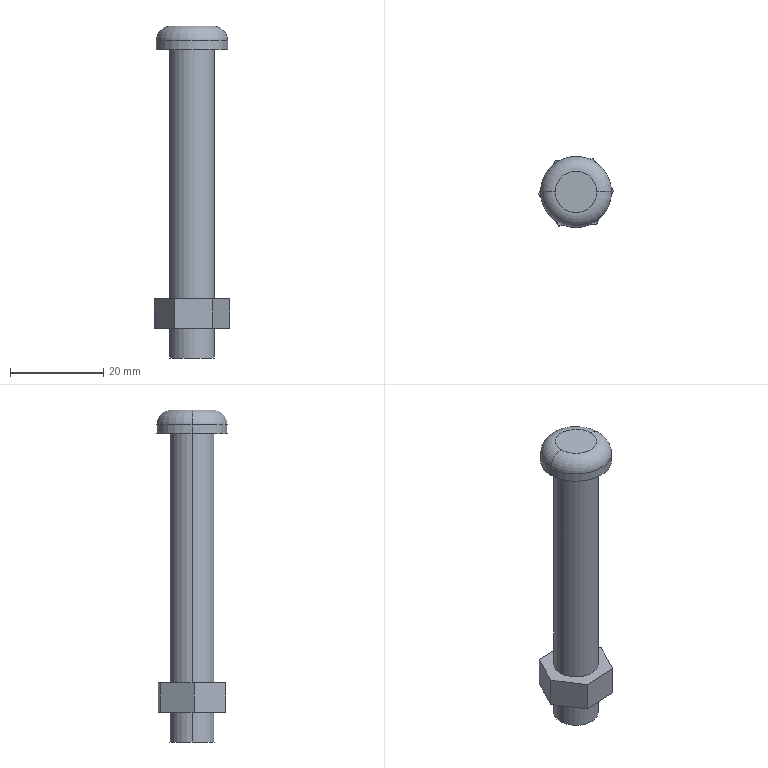Part | SolidWorks | features ICE 2, Extrusion 1, Fillet 1 | 2 solids | 19 faces | box 16.107 x 15.24 x 71.12 mm | volume 6159 mm3 | plane 11 | cylinder 6 | torus 2 | commonest cylinder face diameters 9.525 x4 15.24 x2
STEP:
#1=CARTESIAN_POINT('',(-42.545,-76.2,1.905));
#2=VERTEX_POINT('',#1);
#3=CARTESIAN_POINT('',(-27.305,-76.2,1.905));
#4=VERTEX_POINT('',#3);
#5=CARTESIAN_POINT('',(-34.925,-76.2,1.905));
#6=DIRECTION('',(0.,0.,-1.));
#7=DIRECTION('',(1.,0.,0.));
#8=AXIS2_PLACEMENT_3D('',#5,#6,#7);
#9=CIRCLE('',#8,7.62);
#10=EDGE_CURVE('',#2,#4,#9,.T.);
#11=ORIENTED_EDGE('',*,*,#10,.F.);
#12=CARTESIAN_POINT('',(-39.37,-76.2,5.08));
#13=VERTEX_POINT('',#12);
#14=CARTESIAN_POINT('',(-39.37,-76.2,1.905));
#15=DIRECTION('',(0.,1.,0.));
#16=DIRECTION('',(-1.,0.,0.));
#17=AXIS2_PLACEMENT_3D('',#14,#15,#16);
#18=CIRCLE('',#17,3.175);
#19=EDGE_CURVE('',#2,#13,#18,.T.);
#20=ORIENTED_EDGE('',*,*,#19,.T.);
#21=CARTESIAN_POINT('',(-30.48,-76.2,5.08));
#22=VERTEX_POINT('',#21);
#23=CARTESIAN_POINT('',(-34.925,-76.2,5.08));
#24=DIRECTION('',(0.,0.,1.));
#25=DIRECTION('',(1.,0.,0.));
#26=AXIS2_PLACEMENT_3D('',#23,#24,#25);
#27=CIRCLE('',#26,4.445);
#28=EDGE_CURVE('',#22,#13,#27,.T.);
#29=ORIENTED_EDGE('',*,*,#28,.F.);
#30=CARTESIAN_POINT('',(-30.48,-76.2,1.905));
#31=DIRECTION('',(0.,-1.,0.));
#32=DIRECTION('',(0.,0.,-1.));
#33=AXIS2_PLACEMENT_3D('',#30,#31,#32);
#34=CIRCLE('',#33,3.175);
#35=EDGE_CURVE('',#4,#22,#34,.T.);
#36=ORIENTED_EDGE('',*,*,#35,.F.);
#37=EDGE_LOOP('',(#11,#20,#29,#36));
#38=FACE_OUTER_BOUND('',#37,.T.);
#39=CARTESIAN_POINT('',(-34.925,-76.2,1.905));
#40=DIRECTION('',(0.,0.,1.));
#41=DIRECTION('',(1.,0.,0.));
#42=AXIS2_PLACEMENT_3D('',#39,#40,#41);
#43=TOROIDAL_SURFACE('',#42,4.445,3.175);
#44=ADVANCED_FACE('',(#38),#43,.T.);
#45=ORIENTED_EDGE('',*,*,#10,.T.);
#46=CARTESIAN_POINT('',(-27.305,-76.2,0.));
#47=VERTEX_POINT('',#46);
#48=CARTESIAN_POINT('',(-27.305,-76.2,5.08));
#49=DIRECTION('',(0.,0.,-1.));
#50=VECTOR('',#49,1000.);
#51=LINE('',#48,#50);
#52=EDGE_CURVE('',#4,#47,#51,.T.);
#53=ORIENTED_EDGE('',*,*,#52,.T.);
#54=CARTESIAN_POINT('',(-42.545,-76.2,0.));
#55=VERTEX_POINT('',#54);
#56=CARTESIAN_POINT('',(-34.925,-76.2,0.));
#57=DIRECTION('',(0.,0.,1.));
#58=DIRECTION('',(1.,0.,0.));
#59=AXIS2_PLACEMENT_3D('',#56,#57,#58);
#60=CIRCLE('',#59,7.62);
#61=EDGE_CURVE('',#47,#55,#60,.T.);
#62=ORIENTED_EDGE('',*,*,#61,.T.);
#63=CARTESIAN_POINT('',(-42.545,-76.2,5.08));
#64=DIRECTION('',(0.,0.,-1.));
#65=VECTOR('',#64,1000.);
#66=LINE('',#63,#65);
#67=EDGE_CURVE('',#2,#55,#66,.T.);
#68=ORIENTED_EDGE('',*,*,#67,.F.);
#69=EDGE_LOOP('',(#45,#53,#62,#68));
#70=FACE_OUTER_BOUND('',#69,.T.);
#71=CARTESIAN_POINT('',(-34.925,-76.2,5.08));
#72=DIRECTION('',(0.,0.,-1.));
#73=DIRECTION('',(-1.,0.,0.));
#74=AXIS2_PLACEMENT_3D('',#71,#72,#73);
#75=CYLINDRICAL_SURFACE('',#74,7.62);
#76=ADVANCED_FACE('',(#70),#75,.T.);
#77=CARTESIAN_POINT('',(-39.688,-76.2,-66.04));
#78=VERTEX_POINT('',#77);
#79=CARTESIAN_POINT('',(-30.163,-76.2,-66.04));
#80=VERTEX_POINT('',#79);
#81=CARTESIAN_POINT('',(-34.925,-76.2,-66.04));
#82=DIRECTION('',(0.,0.,-1.));
#83=DIRECTION('',(1.,0.,0.));
#84=AXIS2_PLACEMENT_3D('',#81,#82,#83);
#85=CIRCLE('',#84,4.762);
#86=EDGE_CURVE('',#78,#80,#85,.T.);
#87=ORIENTED_EDGE('',*,*,#86,.F.);
#88=CARTESIAN_POINT('',(-39.688,-76.2,0.));
#89=VERTEX_POINT('',#88);
#90=CARTESIAN_POINT('',(-39.688,-76.2,-92.21));
#91=DIRECTION('',(0.,0.,1.));
#92=VECTOR('',#91,1000.);
#93=LINE('',#90,#92);
#94=EDGE_CURVE('',#78,#89,#93,.T.);
#95=ORIENTED_EDGE('',*,*,#94,.T.);
#96=CARTESIAN_POINT('',(-30.163,-76.2,0.));
#97=VERTEX_POINT('',#96);
#98=CARTESIAN_POINT('',(-34.925,-76.2,0.));
#99=DIRECTION('',(0.,0.,1.));
#100=DIRECTION('',(1.,0.,0.));
#101=AXIS2_PLACEMENT_3D('',#98,#99,#100);
#102=CIRCLE('',#101,4.762);
#103=EDGE_CURVE('',#97,#89,#102,.T.);
#104=ORIENTED_EDGE('',*,*,#103,.F.);
#105=CARTESIAN_POINT('',(-30.163,-76.2,-92.21));
#106=DIRECTION('',(0.,0.,1.));
#107=VECTOR('',#106,1000.);
#108=LINE('',#105,#107);
#109=EDGE_CURVE('',#80,#97,#108,.T.);
#110=ORIENTED_EDGE('',*,*,#109,.F.);
#111=EDGE_LOOP('',(#87,#95,#104,#110));
#112=FACE_OUTER_BOUND('',#111,.T.);
#113=CARTESIAN_POINT('',(-34.925,-76.2,-92.21));
#114=DIRECTION('',(0.,0.,1.));
#115=DIRECTION('',(1.,0.,0.));
#116=AXIS2_PLACEMENT_3D('',#113,#114,#115);
#117=CYLINDRICAL_SURFACE('',#116,4.762);
#118=ADVANCED_FACE('',(#112),#117,.T.);
#119=ORIENTED_EDGE('',*,*,#94,.F.);
#120=CARTESIAN_POINT('',(-34.925,-76.2,-66.04));
#121=DIRECTION('',(0.,0.,-1.));
#122=DIRECTION('',(1.,0.,0.));
#123=AXIS2_PLACEMENT_3D('',#120,#121,#122);
#124=CIRCLE('',#123,4.762);
#125=EDGE_CURVE('',#80,#78,#124,.T.);
#126=ORIENTED_EDGE('',*,*,#125,.F.);
#127=ORIENTED_EDGE('',*,*,#109,.T.);
#128=CARTESIAN_POINT('',(-34.925,-76.2,0.));
#129=DIRECTION('',(0.,0.,1.));
#130=DIRECTION('',(1.,0.,0.));
#131=AXIS2_PLACEMENT_3D('',#128,#129,#130);
#132=CIRCLE('',#131,4.762);
#133=EDGE_CURVE('',#89,#97,#132,.T.);
#134=ORIENTED_EDGE('',*,*,#133,.F.);
#135=EDGE_LOOP('',(#119,#126,#127,#134));
#136=FACE_OUTER_BOUND('',#135,.T.);
#137=CARTESIAN_POINT('',(-34.925,-76.2,-92.21));
#138=DIRECTION('',(0.,0.,1.));
#139=DIRECTION('',(1.,0.,0.));
#140=AXIS2_PLACEMENT_3D('',#137,#138,#139);
#141=CYLINDRICAL_SURFACE('',#140,4.762);
#142=ADVANCED_FACE('',(#136),#141,.T.);
#143=ORIENTED_EDGE('',*,*,#125,.T.);
#144=ORIENTED_EDGE('',*,*,#86,.T.);
#145=EDGE_LOOP('',(#143,#144));
#146=FACE_OUTER_BOUND('',#145,.T.);
#147=CARTESIAN_POINT('',(-66.675,-79.866,-66.04));
#148=DIRECTION('',(0.,0.,1.));
#149=DIRECTION('',(1.,0.,0.));
#150=AXIS2_PLACEMENT_3D('',#147,#148,#149);
#151=PLANE('',#150);
#152=ADVANCED_FACE('',(#146),#151,.F.);
#153=ORIENTED_EDGE('',*,*,#52,.F.);
#154=CARTESIAN_POINT('',(-34.925,-76.2,1.905));
#155=DIRECTION('',(0.,0.,-1.));
#156=DIRECTION('',(1.,0.,0.));
#157=AXIS2_PLACEMENT_3D('',#154,#155,#156);
#158=CIRCLE('',#157,7.62);
#159=EDGE_CURVE('',#4,#2,#158,.T.);
#160=ORIENTED_EDGE('',*,*,#159,.T.);
#161=ORIENTED_EDGE('',*,*,#67,.T.);
#162=CARTESIAN_POINT('',(-34.925,-76.2,0.));
#163=DIRECTION('',(0.,0.,1.));
#164=DIRECTION('',(1.,0.,0.));
#165=AXIS2_PLACEMENT_3D('',#162,#163,#164);
#166=CIRCLE('',#165,7.62);
#167=EDGE_CURVE('',#55,#47,#166,.T.);
#168=ORIENTED_EDGE('',*,*,#167,.T.);
#169=EDGE_LOOP('',(#153,#160,#161,#168));
#170=FACE_OUTER_BOUND('',#169,.T.);
#171=CARTESIAN_POINT('',(-34.925,-76.2,5.08));
#172=DIRECTION('',(0.,0.,-1.));
#173=DIRECTION('',(-1.,0.,0.));
#174=AXIS2_PLACEMENT_3D('',#171,#172,#173);
#175=CYLINDRICAL_SURFACE('',#174,7.62);
#176=ADVANCED_FACE('',(#170),#175,.T.);
#177=ORIENTED_EDGE('',*,*,#28,.T.);
#178=CARTESIAN_POINT('',(-34.925,-76.2,5.08));
#179=DIRECTION('',(0.,0.,1.));
#180=DIRECTION('',(1.,0.,0.));
#181=AXIS2_PLACEMENT_3D('',#178,#179,#180);
#182=CIRCLE('',#181,4.445);
#183=EDGE_CURVE('',#13,#22,#182,.T.);
#184=ORIENTED_EDGE('',*,*,#183,.T.);
#185=EDGE_LOOP('',(#177,#184));
#186=FACE_OUTER_BOUND('',#185,.T.);
#187=CARTESIAN_POINT('',(-34.925,-76.2,5.08));
#188=DIRECTION('',(0.,0.,1.));
#189=DIRECTION('',(1.,0.,0.));
#190=AXIS2_PLACEMENT_3D('',#187,#188,#189);
#191=PLANE('',#190);
#192=ADVANCED_FACE('',(#186),#191,.T.);
#193=ORIENTED_EDGE('',*,*,#103,.T.);
#194=ORIENTED_EDGE('',*,*,#133,.T.);
#195=EDGE_LOOP('',(#193,#194));
#196=FACE_BOUND('',#195,.T.);
#197=ORIENTED_EDGE('',*,*,#167,.F.);
#198=ORIENTED_EDGE('',*,*,#61,.F.);
#199=EDGE_LOOP('',(#197,#198));
#200=FACE_OUTER_BOUND('',#199,.T.);
#201=CARTESIAN_POINT('',(-34.925,-76.2,0.));
#202=DIRECTION('',(0.,0.,1.));
#203=DIRECTION('',(1.,0.,0.));
#204=AXIS2_PLACEMENT_3D('',#201,#202,#203);
#205=PLANE('',#204);
#206=ADVANCED_FACE('',(#196,#200),#205,.F.);
#207=ORIENTED_EDGE('',*,*,#19,.F.);
#208=ORIENTED_EDGE('',*,*,#159,.F.);
#209=ORIENTED_EDGE('',*,*,#35,.T.);
#210=ORIENTED_EDGE('',*,*,#183,.F.);
#211=EDGE_LOOP('',(#207,#208,#209,#210));
#212=FACE_OUTER_BOUND('',#211,.T.);
#213=CARTESIAN_POINT('',(-34.925,-76.2,1.905));
#214=DIRECTION('',(0.,0.,1.));
#215=DIRECTION('',(1.,0.,0.));
#216=AXIS2_PLACEMENT_3D('',#213,#214,#215);
#217=TOROIDAL_SURFACE('',#216,4.445,3.175);
#218=ADVANCED_FACE('',(#212),#217,.T.);
#219=CLOSED_SHELL('',(#44,#76,#118,#142,#152,#176,#192,#206,#218));
#220=MANIFOLD_SOLID_BREP('',#219);
#221=CARTESIAN_POINT('',(-30.163,-76.2,-59.69));
#222=VERTEX_POINT('',#221);
#223=CARTESIAN_POINT('',(-39.688,-76.2,-59.69));
#224=VERTEX_POINT('',#223);
#225=CARTESIAN_POINT('',(-34.925,-76.2,-59.69));
#226=DIRECTION('',(0.,0.,-1.));
#227=DIRECTION('',(-1.,0.,0.));
#228=AXIS2_PLACEMENT_3D('',#225,#226,#227);
#229=CIRCLE('',#228,4.762);
#230=EDGE_CURVE('',#222,#224,#229,.T.);
#231=ORIENTED_EDGE('',*,*,#230,.T.);
#232=CARTESIAN_POINT('',(-39.688,-76.2,-53.34));
#233=VERTEX_POINT('',#232);
#234=CARTESIAN_POINT('',(-39.688,-76.2,-59.69));
#235=DIRECTION('',(0.,0.,1.));
#236=VECTOR('',#235,1000.);
#237=LINE('',#234,#236);
#238=EDGE_CURVE('',#224,#233,#237,.T.);
#239=ORIENTED_EDGE('',*,*,#238,.T.);
#240=CARTESIAN_POINT('',(-30.163,-76.2,-53.34));
#241=VERTEX_POINT('',#240);
#242=CARTESIAN_POINT('',(-34.925,-76.2,-53.34));
#243=DIRECTION('',(0.,0.,-1.));
#244=DIRECTION('',(-1.,0.,0.));
#245=AXIS2_PLACEMENT_3D('',#242,#243,#244);
#246=CIRCLE('',#245,4.762);
#247=EDGE_CURVE('',#241,#233,#246,.T.);
#248=ORIENTED_EDGE('',*,*,#247,.F.);
#249=CARTESIAN_POINT('',(-30.163,-76.2,-59.69));
#250=DIRECTION('',(0.,0.,1.));
#251=VECTOR('',#250,1000.);
#252=LINE('',#249,#251);
#253=EDGE_CURVE('',#222,#241,#252,.T.);
#254=ORIENTED_EDGE('',*,*,#253,.F.);
#255=EDGE_LOOP('',(#231,#239,#248,#254));
#256=FACE_OUTER_BOUND('',#255,.T.);
#257=CARTESIAN_POINT('',(-34.925,-76.2,-59.69));
#258=DIRECTION('',(0.,0.,1.));
#259=DIRECTION('',(1.,0.,0.));
#260=AXIS2_PLACEMENT_3D('',#257,#258,#259);
#261=CYLINDRICAL_SURFACE('',#260,4.762);
#262=ADVANCED_FACE('',(#256),#261,.F.);
#263=CARTESIAN_POINT('',(-42.979,-76.638,-59.69));
#264=VERTEX_POINT('',#263);
#265=CARTESIAN_POINT('',(-39.331,-69.444,-59.69));
#266=VERTEX_POINT('',#265);
#267=CARTESIAN_POINT('',(-42.979,-76.638,-59.69));
#268=DIRECTION('',(0.4522,0.8919,0.));
#269=VECTOR('',#268,1000.);
#270=LINE('',#267,#269);
#271=EDGE_CURVE('',#264,#266,#270,.T.);
#272=ORIENTED_EDGE('',*,*,#271,.T.);
#273=CARTESIAN_POINT('',(-31.278,-69.006,-59.69));
#274=VERTEX_POINT('',#273);
#275=CARTESIAN_POINT('',(-39.331,-69.444,-59.69));
#276=DIRECTION('',(0.9985,0.05432,0.));
#277=VECTOR('',#276,1000.);
#278=LINE('',#275,#277);
#279=EDGE_CURVE('',#266,#274,#278,.T.);
#280=ORIENTED_EDGE('',*,*,#279,.T.);
#281=CARTESIAN_POINT('',(-26.871,-75.762,-59.69));
#282=VERTEX_POINT('',#281);
#283=CARTESIAN_POINT('',(-31.278,-69.006,-59.69));
#284=DIRECTION('',(0.5463,-0.8376,0.));
#285=VECTOR('',#284,1000.);
#286=LINE('',#283,#285);
#287=EDGE_CURVE('',#274,#282,#286,.T.);
#288=ORIENTED_EDGE('',*,*,#287,.T.);
#289=CARTESIAN_POINT('',(-30.519,-82.956,-59.69));
#290=VERTEX_POINT('',#289);
#291=CARTESIAN_POINT('',(-26.871,-75.762,-59.69));
#292=DIRECTION('',(-0.4522,-0.8919,0.));
#293=VECTOR('',#292,1000.);
#294=LINE('',#291,#293);
#295=EDGE_CURVE('',#282,#290,#294,.T.);
#296=ORIENTED_EDGE('',*,*,#295,.T.);
#297=CARTESIAN_POINT('',(-38.572,-83.394,-59.69));
#298=VERTEX_POINT('',#297);
#299=CARTESIAN_POINT('',(-30.519,-82.956,-59.69));
#300=DIRECTION('',(-0.9985,-0.05432,0.));
#301=VECTOR('',#300,1000.);
#302=LINE('',#299,#301);
#303=EDGE_CURVE('',#290,#298,#302,.T.);
#304=ORIENTED_EDGE('',*,*,#303,.T.);
#305=CARTESIAN_POINT('',(-38.572,-83.394,-59.69));
#306=DIRECTION('',(-0.5463,0.8376,0.));
#307=VECTOR('',#306,1000.);
#308=LINE('',#305,#307);
#309=EDGE_CURVE('',#298,#264,#308,.T.);
#310=ORIENTED_EDGE('',*,*,#309,.T.);
#311=EDGE_LOOP('',(#272,#280,#288,#296,#304,#310));
#312=FACE_OUTER_BOUND('',#311,.T.);
#313=ORIENTED_EDGE('',*,*,#230,.F.);
#314=CARTESIAN_POINT('',(-34.925,-76.2,-59.69));
#315=DIRECTION('',(0.,0.,-1.));
#316=DIRECTION('',(-1.,0.,0.));
#317=AXIS2_PLACEMENT_3D('',#314,#315,#316);
#318=CIRCLE('',#317,4.762);
#319=EDGE_CURVE('',#224,#222,#318,.T.);
#320=ORIENTED_EDGE('',*,*,#319,.F.);
#321=EDGE_LOOP('',(#313,#320));
#322=FACE_BOUND('',#321,.T.);
#323=CARTESIAN_POINT('',(0.,0.,-59.69));
#324=DIRECTION('',(0.,0.,-1.));
#325=DIRECTION('',(-1.,0.,0.));
#326=AXIS2_PLACEMENT_3D('',#323,#324,#325);
#327=PLANE('',#326);
#328=ADVANCED_FACE('',(#312,#322),#327,.T.);
#329=CARTESIAN_POINT('',(-42.979,-76.638,-53.34));
#330=VERTEX_POINT('',#329);
#331=CARTESIAN_POINT('',(-39.331,-69.444,-53.34));
#332=VERTEX_POINT('',#331);
#333=CARTESIAN_POINT('',(-42.979,-76.638,-53.34));
#334=DIRECTION('',(0.4522,0.8919,0.));
#335=VECTOR('',#334,1000.);
#336=LINE('',#333,#335);
#337=EDGE_CURVE('',#330,#332,#336,.T.);
#338=ORIENTED_EDGE('',*,*,#337,.F.);
#339=CARTESIAN_POINT('',(-38.572,-83.394,-53.34));
#340=VERTEX_POINT('',#339);
#341=CARTESIAN_POINT('',(-38.572,-83.394,-53.34));
#342=DIRECTION('',(-0.5463,0.8376,0.));
#343=VECTOR('',#342,1000.);
#344=LINE('',#341,#343);
#345=EDGE_CURVE('',#340,#330,#344,.T.);
#346=ORIENTED_EDGE('',*,*,#345,.F.);
#347=CARTESIAN_POINT('',(-30.519,-82.956,-53.34));
#348=VERTEX_POINT('',#347);
#349=CARTESIAN_POINT('',(-30.519,-82.956,-53.34));
#350=DIRECTION('',(-0.9985,-0.05432,0.));
#351=VECTOR('',#350,1000.);
#352=LINE('',#349,#351);
#353=EDGE_CURVE('',#348,#340,#352,.T.);
#354=ORIENTED_EDGE('',*,*,#353,.F.);
#355=CARTESIAN_POINT('',(-26.871,-75.762,-53.34));
#356=VERTEX_POINT('',#355);
#357=CARTESIAN_POINT('',(-26.871,-75.762,-53.34));
#358=DIRECTION('',(-0.4522,-0.8919,0.));
#359=VECTOR('',#358,1000.);
#360=LINE('',#357,#359);
#361=EDGE_CURVE('',#356,#348,#360,.T.);
#362=ORIENTED_EDGE('',*,*,#361,.F.);
#363=CARTESIAN_POINT('',(-31.278,-69.006,-53.34));
#364=VERTEX_POINT('',#363);
#365=CARTESIAN_POINT('',(-31.278,-69.006,-53.34));
#366=DIRECTION('',(0.5463,-0.8376,0.));
#367=VECTOR('',#366,1000.);
#368=LINE('',#365,#367);
#369=EDGE_CURVE('',#364,#356,#368,.T.);
#370=ORIENTED_EDGE('',*,*,#369,.F.);
#371=CARTESIAN_POINT('',(-39.331,-69.444,-53.34));
#372=DIRECTION('',(0.9985,0.05432,0.));
#373=VECTOR('',#372,1000.);
#374=LINE('',#371,#373);
#375=EDGE_CURVE('',#332,#364,#374,.T.);
#376=ORIENTED_EDGE('',*,*,#375,.F.);
#377=EDGE_LOOP('',(#338,#346,#354,#362,#370,#376));
#378=FACE_OUTER_BOUND('',#377,.T.);
#379=ORIENTED_EDGE('',*,*,#247,.T.);
#380=CARTESIAN_POINT('',(-34.925,-76.2,-53.34));
#381=DIRECTION('',(0.,0.,-1.));
#382=DIRECTION('',(-1.,0.,0.));
#383=AXIS2_PLACEMENT_3D('',#380,#381,#382);
#384=CIRCLE('',#383,4.762);
#385=EDGE_CURVE('',#233,#241,#384,.T.);
#386=ORIENTED_EDGE('',*,*,#385,.T.);
#387=EDGE_LOOP('',(#379,#386));
#388=FACE_BOUND('',#387,.T.);
#389=CARTESIAN_POINT('',(0.,0.,-53.34));
#390=DIRECTION('',(0.,0.,-1.));
#391=DIRECTION('',(-1.,0.,0.));
#392=AXIS2_PLACEMENT_3D('',#389,#390,#391);
#393=PLANE('',#392);
#394=ADVANCED_FACE('',(#378,#388),#393,.F.);
#395=ORIENTED_EDGE('',*,*,#337,.T.);
#396=CARTESIAN_POINT('',(-39.331,-69.444,-59.69));
#397=DIRECTION('',(0.,0.,1.));
#398=VECTOR('',#397,1000.);
#399=LINE('',#396,#398);
#400=EDGE_CURVE('',#266,#332,#399,.T.);
#401=ORIENTED_EDGE('',*,*,#400,.F.);
#402=ORIENTED_EDGE('',*,*,#271,.F.);
#403=CARTESIAN_POINT('',(-42.979,-76.638,-59.69));
#404=DIRECTION('',(0.,0.,1.));
#405=VECTOR('',#404,1000.);
#406=LINE('',#403,#405);
#407=EDGE_CURVE('',#264,#330,#406,.T.);
#408=ORIENTED_EDGE('',*,*,#407,.T.);
#409=EDGE_LOOP('',(#395,#401,#402,#408));
#410=FACE_OUTER_BOUND('',#409,.T.);
#411=CARTESIAN_POINT('',(-42.979,-76.638,-59.69));
#412=DIRECTION('',(0.8919,-0.4522,0.));
#413=DIRECTION('',(0.4522,0.8919,0.));
#414=AXIS2_PLACEMENT_3D('',#411,#412,#413);
#415=PLANE('',#414);
#416=ADVANCED_FACE('',(#410),#415,.F.);
#417=ORIENTED_EDGE('',*,*,#375,.T.);
#418=CARTESIAN_POINT('',(-31.278,-69.006,-59.69));
#419=DIRECTION('',(0.,0.,1.));
#420=VECTOR('',#419,1000.);
#421=LINE('',#418,#420);
#422=EDGE_CURVE('',#274,#364,#421,.T.);
#423=ORIENTED_EDGE('',*,*,#422,.F.);
#424=ORIENTED_EDGE('',*,*,#279,.F.);
#425=ORIENTED_EDGE('',*,*,#400,.T.);
#426=EDGE_LOOP('',(#417,#423,#424,#425));
#427=FACE_OUTER_BOUND('',#426,.T.);
#428=CARTESIAN_POINT('',(-39.331,-69.444,-59.69));
#429=DIRECTION('',(0.05432,-0.9985,0.));
#430=DIRECTION('',(0.9985,0.05432,0.));
#431=AXIS2_PLACEMENT_3D('',#428,#429,#430);
#432=PLANE('',#431);
#433=ADVANCED_FACE('',(#427),#432,.F.);
#434=ORIENTED_EDGE('',*,*,#369,.T.);
#435=CARTESIAN_POINT('',(-26.871,-75.762,-59.69));
#436=DIRECTION('',(0.,0.,1.));
#437=VECTOR('',#436,1000.);
#438=LINE('',#435,#437);
#439=EDGE_CURVE('',#282,#356,#438,.T.);
#440=ORIENTED_EDGE('',*,*,#439,.F.);
#441=ORIENTED_EDGE('',*,*,#287,.F.);
#442=ORIENTED_EDGE('',*,*,#422,.T.);
#443=EDGE_LOOP('',(#434,#440,#441,#442));
#444=FACE_OUTER_BOUND('',#443,.T.);
#445=CARTESIAN_POINT('',(-31.278,-69.006,-59.69));
#446=DIRECTION('',(-0.8376,-0.5463,0.));
#447=DIRECTION('',(0.5463,-0.8376,0.));
#448=AXIS2_PLACEMENT_3D('',#445,#446,#447);
#449=PLANE('',#448);
#450=ADVANCED_FACE('',(#444),#449,.F.);
#451=ORIENTED_EDGE('',*,*,#361,.T.);
#452=CARTESIAN_POINT('',(-30.519,-82.956,-59.69));
#453=DIRECTION('',(0.,0.,1.));
#454=VECTOR('',#453,1000.);
#455=LINE('',#452,#454);
#456=EDGE_CURVE('',#290,#348,#455,.T.);
#457=ORIENTED_EDGE('',*,*,#456,.F.);
#458=ORIENTED_EDGE('',*,*,#295,.F.);
#459=ORIENTED_EDGE('',*,*,#439,.T.);
#460=EDGE_LOOP('',(#451,#457,#458,#459));
#461=FACE_OUTER_BOUND('',#460,.T.);
#462=CARTESIAN_POINT('',(-26.871,-75.762,-59.69));
#463=DIRECTION('',(-0.8919,0.4522,0.));
#464=DIRECTION('',(-0.4522,-0.8919,0.));
#465=AXIS2_PLACEMENT_3D('',#462,#463,#464);
#466=PLANE('',#465);
#467=ADVANCED_FACE('',(#461),#466,.F.);
#468=ORIENTED_EDGE('',*,*,#353,.T.);
#469=CARTESIAN_POINT('',(-38.572,-83.394,-59.69));
#470=DIRECTION('',(0.,0.,1.));
#471=VECTOR('',#470,1000.);
#472=LINE('',#469,#471);
#473=EDGE_CURVE('',#298,#340,#472,.T.);
#474=ORIENTED_EDGE('',*,*,#473,.F.);
#475=ORIENTED_EDGE('',*,*,#303,.F.);
#476=ORIENTED_EDGE('',*,*,#456,.T.);
#477=EDGE_LOOP('',(#468,#474,#475,#476));
#478=FACE_OUTER_BOUND('',#477,.T.);
#479=CARTESIAN_POINT('',(-30.519,-82.956,-59.69));
#480=DIRECTION('',(-0.05432,0.9985,0.));
#481=DIRECTION('',(-0.9985,-0.05432,0.));
#482=AXIS2_PLACEMENT_3D('',#479,#480,#481);
#483=PLANE('',#482);
#484=ADVANCED_FACE('',(#478),#483,.F.);
#485=ORIENTED_EDGE('',*,*,#345,.T.);
#486=ORIENTED_EDGE('',*,*,#407,.F.);
#487=ORIENTED_EDGE('',*,*,#309,.F.);
#488=ORIENTED_EDGE('',*,*,#473,.T.);
#489=EDGE_LOOP('',(#485,#486,#487,#488));
#490=FACE_OUTER_BOUND('',#489,.T.);
#491=CARTESIAN_POINT('',(-38.572,-83.394,-59.69));
#492=DIRECTION('',(0.8376,0.5463,0.));
#493=DIRECTION('',(-0.5463,0.8376,0.));
#494=AXIS2_PLACEMENT_3D('',#491,#492,#493);
#495=PLANE('',#494);
#496=ADVANCED_FACE('',(#490),#495,.F.);
#497=ORIENTED_EDGE('',*,*,#238,.F.);
#498=ORIENTED_EDGE('',*,*,#319,.T.);
#499=ORIENTED_EDGE('',*,*,#253,.T.);
#500=ORIENTED_EDGE('',*,*,#385,.F.);
#501=EDGE_LOOP('',(#497,#498,#499,#500));
#502=FACE_OUTER_BOUND('',#501,.T.);
#503=CARTESIAN_POINT('',(-34.925,-76.2,-59.69));
#504=DIRECTION('',(0.,0.,1.));
#505=DIRECTION('',(1.,0.,0.));
#506=AXIS2_PLACEMENT_3D('',#503,#504,#505);
#507=CYLINDRICAL_SURFACE('',#506,4.762);
#508=ADVANCED_FACE('',(#502),#507,.F.);
#509=CLOSED_SHELL('',(#262,#328,#394,#416,#433,#450,#467,#484,#496,#508));
#510=MANIFOLD_SOLID_BREP('',#509);
#511=CARTESIAN_POINT('',(0.,0.,0.));
#512=DIRECTION('',(0.,0.,1.));
#513=DIRECTION('',(1.,0.,0.));
#514=AXIS2_PLACEMENT_3D('',#511,#512,#513);
#515=(LENGTH_UNIT()NAMED_UNIT(*)SI_UNIT(.MILLI.,.METRE.));
#516=UNCERTAINTY_MEASURE_WITH_UNIT(LENGTH_MEASURE(0.00001),#515,'','');
#517=(NAMED_UNIT(*)PLANE_ANGLE_UNIT()SI_UNIT($,.RADIAN.));
#518=(NAMED_UNIT(*)SI_UNIT($,.STERADIAN.)SOLID_ANGLE_UNIT());
#519=(GEOMETRIC_REPRESENTATION_CONTEXT(3)GLOBAL_UNCERTAINTY_ASSIGNED_CONTEXT((#516))GLOBAL_UNIT_ASSIGNED_CONTEXT((#515,#517,#518))REPRESENTATION_CONTEXT('',''));
#520=ADVANCED_BREP_SHAPE_REPRESENTATION('',(#220,#510,#514),#519);